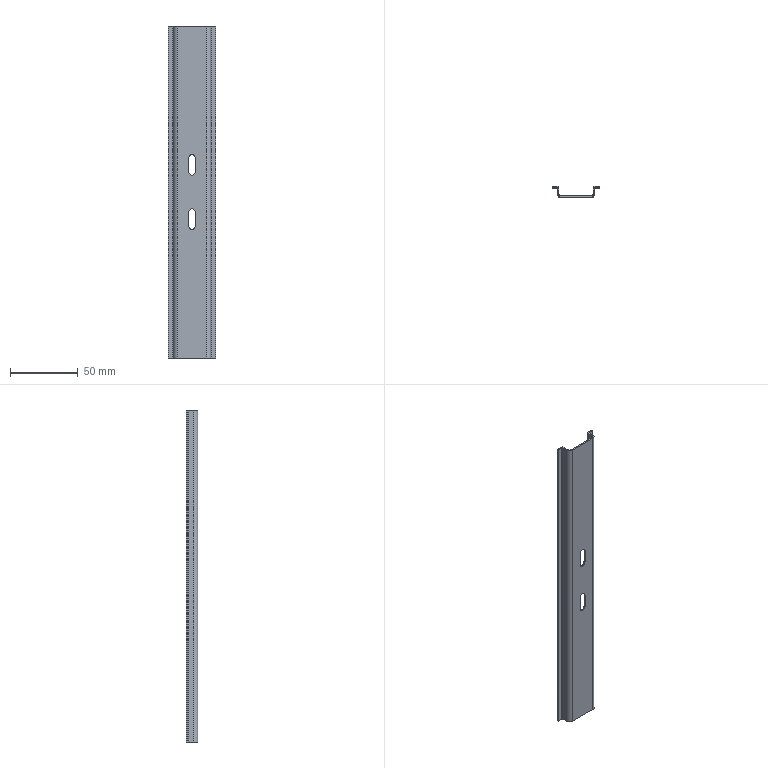Part | STEP file | Guide rail L_L245 | 1 solid | 30 faces | box 35 x 8.3 x 245 mm | volume 11487 mm3 | plane 18 | cylinder 12 | commonest cylinder face diameters 1 x4 5 x4 4 x2 6 x2